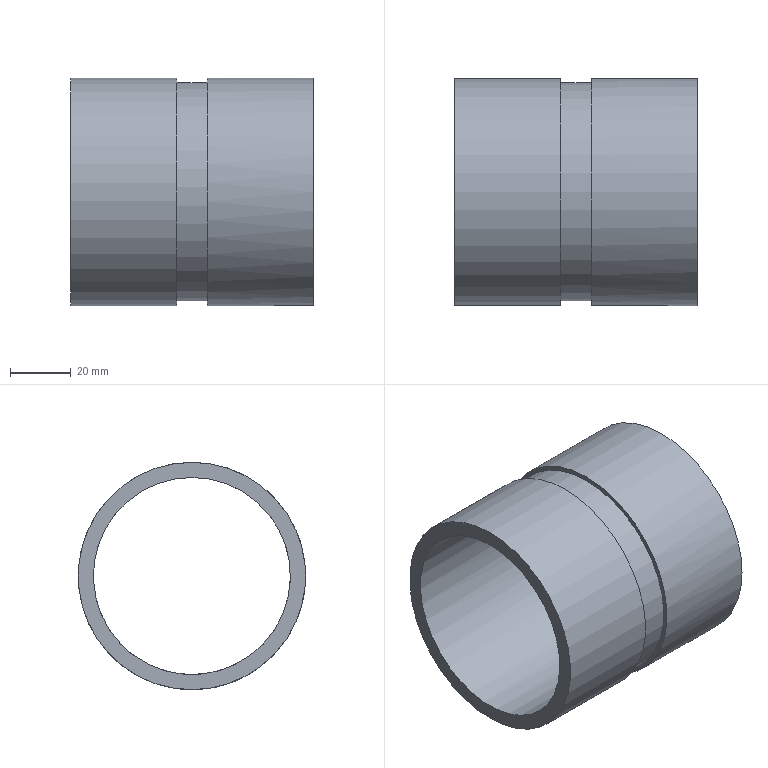Part | STEP file | gslz 2016.10.28-13_id442_x_t | 1 solid | 8 faces | box 80 x 75 x 75 mm | volume 84501 mm3 | cylinder 4 | plane 4 | commonest cylinder face diameters 75 x2 65 x1 72 x1
STEP:
#1=CARTESIAN_POINT('',(0.,0.,0.));
#2=DIRECTION('',(0.,0.,1.));
#3=DIRECTION('',(1.,0.,0.));
#4=AXIS2_PLACEMENT_3D('',#1,#2,#3);
#5=CARTESIAN_POINT('',(-1095.,-690.,260.5));
#6=VERTEX_POINT('',#5);
#7=CARTESIAN_POINT('',(-1095.,-690.,223.));
#8=DIRECTION('',(-1.,0.,0.));
#9=DIRECTION('',(0.,0.,1.));
#10=AXIS2_PLACEMENT_3D('',#7,#8,#9);
#11=CIRCLE('',#10,37.5);
#12=CARTESIAN_POINT('',(-1140.,-690.,223.));
#13=DIRECTION('',(1.,0.,0.));
#14=DIRECTION('',(0.,0.,1.));
#15=AXIS2_PLACEMENT_3D('',#12,#13,#14);
#16=CYLINDRICAL_SURFACE('',#15,37.5);
#17=CARTESIAN_POINT('',(6.283,45.));
#18=DIRECTION('',(-1.,0.));
#19=VECTOR('',#18,1.);
#20=LINE('',#17,#19);
#21=(GEOMETRIC_REPRESENTATION_CONTEXT(2)PARAMETRIC_REPRESENTATION_CONTEXT()REPRESENTATION_CONTEXT('',''));
#22=DEFINITIONAL_REPRESENTATION('',(#20),#21);
#23=PCURVE('',#16,#22);
#24=CARTESIAN_POINT('',(-1095.,-690.,223.));
#25=DIRECTION('',(1.,0.,0.));
#26=DIRECTION('',(0.,0.,1.));
#27=AXIS2_PLACEMENT_3D('',#24,#25,#26);
#28=PLANE('',#27);
#29=CARTESIAN_POINT('',(37.5,0.));
#30=CARTESIAN_POINT('',(37.5,-64.952));
#31=CARTESIAN_POINT('',(-18.75,-32.476));
#32=CARTESIAN_POINT('',(-75.,0.));
#33=CARTESIAN_POINT('',(-18.75,32.476));
#34=CARTESIAN_POINT('',(37.5,64.952));
#35=CARTESIAN_POINT('',(37.5,0.));
#36=(BOUNDED_CURVE()B_SPLINE_CURVE(2,(#29,#30,#31,#32,#33,#34,#35),.UNSPECIFIED.,.T.,.F.)B_SPLINE_CURVE_WITH_KNOTS((1,2,2,2,2,1),(-2.094,0.,2.094,4.189,6.283,8.378),.UNSPECIFIED.)CURVE()GEOMETRIC_REPRESENTATION_ITEM()RATIONAL_B_SPLINE_CURVE((1.,0.5,1.,0.5,1.,0.5,1.))REPRESENTATION_ITEM(''));
#37=(GEOMETRIC_REPRESENTATION_CONTEXT(2)PARAMETRIC_REPRESENTATION_CONTEXT()REPRESENTATION_CONTEXT('',''));
#38=DEFINITIONAL_REPRESENTATION('',(#36),#37);
#39=PCURVE('',#28,#38);
#40=SURFACE_CURVE('',#11,(#23,#39),.PCURVE_S1.);
#41=EDGE_CURVE('',#6,#6,#40,.T.);
#42=ORIENTED_EDGE('',*,*,#41,.F.);
#43=CARTESIAN_POINT('',(-1060.,-690.,260.5));
#44=VERTEX_POINT('',#43);
#45=CARTESIAN_POINT('',(-1095.,-690.,260.5));
#46=CARTESIAN_POINT('',(-1060.,-690.,260.5));
#47=B_SPLINE_CURVE_WITH_KNOTS('',1,(#45,#46),.UNSPECIFIED.,.F.,.F.,(2,2),(45.,80.),.PIECEWISE_BEZIER_KNOTS.);
#48=CARTESIAN_POINT('',(6.283,0.));
#49=DIRECTION('',(0.,1.));
#50=VECTOR('',#49,1.);
#51=LINE('',#48,#50);
#52=(GEOMETRIC_REPRESENTATION_CONTEXT(2)PARAMETRIC_REPRESENTATION_CONTEXT()REPRESENTATION_CONTEXT('',''));
#53=DEFINITIONAL_REPRESENTATION('',(#51),#52);
#54=PCURVE('',#16,#53);
#55=CARTESIAN_POINT('',(0.,0.));
#56=DIRECTION('',(0.,1.));
#57=VECTOR('',#56,1.);
#58=LINE('',#55,#57);
#59=(GEOMETRIC_REPRESENTATION_CONTEXT(2)PARAMETRIC_REPRESENTATION_CONTEXT()REPRESENTATION_CONTEXT('',''));
#60=DEFINITIONAL_REPRESENTATION('',(#58),#59);
#61=PCURVE('',#16,#60);
#62=SEAM_CURVE('',#47,(#54,#61),.PCURVE_S1.);
#63=EDGE_CURVE('',#6,#44,#62,.T.);
#64=ORIENTED_EDGE('',*,*,#63,.T.);
#65=CARTESIAN_POINT('',(-1060.,-727.5,223.));
#66=VERTEX_POINT('',#65);
#67=CARTESIAN_POINT('',(-1060.,-690.,223.));
#68=DIRECTION('',(-1.,0.,0.));
#69=DIRECTION('',(0.,-1.,0.));
#70=AXIS2_PLACEMENT_3D('',#67,#68,#69);
#71=CIRCLE('',#70,37.5);
#72=CARTESIAN_POINT('',(7.854,80.));
#73=DIRECTION('',(-1.,0.));
#74=VECTOR('',#73,1.);
#75=LINE('',#72,#74);
#76=(GEOMETRIC_REPRESENTATION_CONTEXT(2)PARAMETRIC_REPRESENTATION_CONTEXT()REPRESENTATION_CONTEXT('',''));
#77=DEFINITIONAL_REPRESENTATION('',(#75),#76);
#78=PCURVE('',#16,#77);
#79=CARTESIAN_POINT('',(-1060.,-585.,179.));
#80=DIRECTION('',(-1.,0.,0.));
#81=DIRECTION('',(0.,1.,0.));
#82=AXIS2_PLACEMENT_3D('',#79,#80,#81);
#83=PLANE('',#82);
#84=CARTESIAN_POINT('',(-105.,-44.));
#85=DIRECTION('',(-1.,0.));
#86=AXIS2_PLACEMENT_2D('',#84,#85);
#87=CIRCLE('',#86,37.5);
#88=(GEOMETRIC_REPRESENTATION_CONTEXT(2)PARAMETRIC_REPRESENTATION_CONTEXT()REPRESENTATION_CONTEXT('',''));
#89=DEFINITIONAL_REPRESENTATION('',(#87),#88);
#90=PCURVE('',#83,#89);
#91=SURFACE_CURVE('',#71,(#78,#90),.PCURVE_S1.);
#92=EDGE_CURVE('',#44,#66,#91,.T.);
#93=ORIENTED_EDGE('',*,*,#92,.T.);
#94=CARTESIAN_POINT('',(-1060.,-690.,223.));
#95=DIRECTION('',(-1.,0.,0.));
#96=DIRECTION('',(0.,-1.,0.));
#97=AXIS2_PLACEMENT_3D('',#94,#95,#96);
#98=CIRCLE('',#97,37.5);
#99=CARTESIAN_POINT('',(1.571,80.));
#100=DIRECTION('',(-1.,0.));
#101=VECTOR('',#100,1.);
#102=LINE('',#99,#101);
#103=(GEOMETRIC_REPRESENTATION_CONTEXT(2)PARAMETRIC_REPRESENTATION_CONTEXT()REPRESENTATION_CONTEXT('',''));
#104=DEFINITIONAL_REPRESENTATION('',(#102),#103);
#105=PCURVE('',#16,#104);
#106=CARTESIAN_POINT('',(-105.,-44.));
#107=DIRECTION('',(-1.,0.));
#108=AXIS2_PLACEMENT_2D('',#106,#107);
#109=CIRCLE('',#108,37.5);
#110=(GEOMETRIC_REPRESENTATION_CONTEXT(2)PARAMETRIC_REPRESENTATION_CONTEXT()REPRESENTATION_CONTEXT('',''));
#111=DEFINITIONAL_REPRESENTATION('',(#109),#110);
#112=PCURVE('',#83,#111);
#113=SURFACE_CURVE('',#98,(#105,#112),.PCURVE_S1.);
#114=EDGE_CURVE('',#66,#44,#113,.T.);
#115=ORIENTED_EDGE('',*,*,#114,.T.);
#116=ORIENTED_EDGE('',*,*,#63,.F.);
#117=EDGE_LOOP('',(#42,#64,#93,#115,#116));
#118=FACE_BOUND('',#117,.T.);
#119=ADVANCED_FACE('',(#118),#16,.T.);
#120=CARTESIAN_POINT('',(-1060.,-722.5,223.));
#121=VERTEX_POINT('',#120);
#122=CARTESIAN_POINT('',(-1060.,-690.,255.5));
#123=VERTEX_POINT('',#122);
#124=CARTESIAN_POINT('',(-1060.,-690.,223.));
#125=DIRECTION('',(-1.,0.,0.));
#126=DIRECTION('',(0.,-1.,0.));
#127=AXIS2_PLACEMENT_3D('',#124,#125,#126);
#128=CIRCLE('',#127,32.5);
#129=CARTESIAN_POINT('',(-105.,-44.));
#130=DIRECTION('',(-1.,0.));
#131=AXIS2_PLACEMENT_2D('',#129,#130);
#132=CIRCLE('',#131,32.5);
#133=(GEOMETRIC_REPRESENTATION_CONTEXT(2)PARAMETRIC_REPRESENTATION_CONTEXT()REPRESENTATION_CONTEXT('',''));
#134=DEFINITIONAL_REPRESENTATION('',(#132),#133);
#135=PCURVE('',#83,#134);
#136=CARTESIAN_POINT('',(-1140.,-690.,223.));
#137=DIRECTION('',(1.,0.,0.));
#138=DIRECTION('',(0.,0.,1.));
#139=AXIS2_PLACEMENT_3D('',#136,#137,#138);
#140=CYLINDRICAL_SURFACE('',#139,32.5);
#141=CARTESIAN_POINT('',(1.571,80.));
#142=DIRECTION('',(-1.,0.));
#143=VECTOR('',#142,1.);
#144=LINE('',#141,#143);
#145=(GEOMETRIC_REPRESENTATION_CONTEXT(2)PARAMETRIC_REPRESENTATION_CONTEXT()REPRESENTATION_CONTEXT('',''));
#146=DEFINITIONAL_REPRESENTATION('',(#144),#145);
#147=PCURVE('',#140,#146);
#148=SURFACE_CURVE('',#128,(#135,#147),.PCURVE_S1.);
#149=EDGE_CURVE('',#121,#123,#148,.T.);
#150=ORIENTED_EDGE('',*,*,#149,.T.);
#151=CARTESIAN_POINT('',(-1060.,-690.,223.));
#152=DIRECTION('',(-1.,0.,0.));
#153=DIRECTION('',(0.,-1.,0.));
#154=AXIS2_PLACEMENT_3D('',#151,#152,#153);
#155=CIRCLE('',#154,32.5);
#156=CARTESIAN_POINT('',(-105.,-44.));
#157=DIRECTION('',(-1.,0.));
#158=AXIS2_PLACEMENT_2D('',#156,#157);
#159=CIRCLE('',#158,32.5);
#160=(GEOMETRIC_REPRESENTATION_CONTEXT(2)PARAMETRIC_REPRESENTATION_CONTEXT()REPRESENTATION_CONTEXT('',''));
#161=DEFINITIONAL_REPRESENTATION('',(#159),#160);
#162=PCURVE('',#83,#161);
#163=CARTESIAN_POINT('',(7.854,80.));
#164=DIRECTION('',(-1.,0.));
#165=VECTOR('',#164,1.);
#166=LINE('',#163,#165);
#167=(GEOMETRIC_REPRESENTATION_CONTEXT(2)PARAMETRIC_REPRESENTATION_CONTEXT()REPRESENTATION_CONTEXT('',''));
#168=DEFINITIONAL_REPRESENTATION('',(#166),#167);
#169=PCURVE('',#140,#168);
#170=SURFACE_CURVE('',#155,(#162,#169),.PCURVE_S1.);
#171=EDGE_CURVE('',#123,#121,#170,.T.);
#172=ORIENTED_EDGE('',*,*,#171,.T.);
#173=EDGE_LOOP('',(#150,#172));
#174=FACE_BOUND('',#173,.T.);
#175=ORIENTED_EDGE('',*,*,#114,.F.);
#176=ORIENTED_EDGE('',*,*,#92,.F.);
#177=EDGE_LOOP('',(#175,#176));
#178=FACE_BOUND('',#177,.T.);
#179=ADVANCED_FACE('',(#174,#178),#83,.F.);
#180=CARTESIAN_POINT('',(-1140.,-690.,255.5));
#181=VERTEX_POINT('',#180);
#182=CARTESIAN_POINT('',(-1140.,-690.,223.));
#183=DIRECTION('',(1.,0.,0.));
#184=DIRECTION('',(0.,0.,1.));
#185=AXIS2_PLACEMENT_3D('',#182,#183,#184);
#186=CIRCLE('',#185,32.5);
#187=CARTESIAN_POINT('',(-1140.,-690.,223.));
#188=DIRECTION('',(-1.,0.,0.));
#189=DIRECTION('',(0.,0.,-1.));
#190=AXIS2_PLACEMENT_3D('',#187,#188,#189);
#191=PLANE('',#190);
#192=CARTESIAN_POINT('',(-32.5,0.));
#193=CARTESIAN_POINT('',(-32.5,56.292));
#194=CARTESIAN_POINT('',(16.25,28.146));
#195=CARTESIAN_POINT('',(65.,0.));
#196=CARTESIAN_POINT('',(16.25,-28.146));
#197=CARTESIAN_POINT('',(-32.5,-56.292));
#198=CARTESIAN_POINT('',(-32.5,0.));
#199=(BOUNDED_CURVE()B_SPLINE_CURVE(2,(#192,#193,#194,#195,#196,#197,#198),.UNSPECIFIED.,.T.,.F.)B_SPLINE_CURVE_WITH_KNOTS((1,2,2,2,2,1),(-2.094,0.,2.094,4.189,6.283,8.378),.UNSPECIFIED.)CURVE()GEOMETRIC_REPRESENTATION_ITEM()RATIONAL_B_SPLINE_CURVE((1.,0.5,1.,0.5,1.,0.5,1.))REPRESENTATION_ITEM(''));
#200=(GEOMETRIC_REPRESENTATION_CONTEXT(2)PARAMETRIC_REPRESENTATION_CONTEXT()REPRESENTATION_CONTEXT('',''));
#201=DEFINITIONAL_REPRESENTATION('',(#199),#200);
#202=PCURVE('',#191,#201);
#203=CARTESIAN_POINT('',(0.,0.));
#204=DIRECTION('',(1.,0.));
#205=VECTOR('',#204,1.);
#206=LINE('',#203,#205);
#207=(GEOMETRIC_REPRESENTATION_CONTEXT(2)PARAMETRIC_REPRESENTATION_CONTEXT()REPRESENTATION_CONTEXT('',''));
#208=DEFINITIONAL_REPRESENTATION('',(#206),#207);
#209=PCURVE('',#140,#208);
#210=SURFACE_CURVE('',#186,(#202,#209),.PCURVE_S1.);
#211=EDGE_CURVE('',#181,#181,#210,.T.);
#212=ORIENTED_EDGE('',*,*,#211,.T.);
#213=EDGE_LOOP('',(#212));
#214=FACE_BOUND('',#213,.T.);
#215=CARTESIAN_POINT('',(-1140.,-690.,260.5));
#216=VERTEX_POINT('',#215);
#217=CARTESIAN_POINT('',(-1140.,-690.,223.));
#218=DIRECTION('',(1.,0.,0.));
#219=DIRECTION('',(0.,0.,1.));
#220=AXIS2_PLACEMENT_3D('',#217,#218,#219);
#221=CIRCLE('',#220,37.5);
#222=CARTESIAN_POINT('',(-37.5,0.));
#223=CARTESIAN_POINT('',(-37.5,64.952));
#224=CARTESIAN_POINT('',(18.75,32.476));
#225=CARTESIAN_POINT('',(75.,0.));
#226=CARTESIAN_POINT('',(18.75,-32.476));
#227=CARTESIAN_POINT('',(-37.5,-64.952));
#228=CARTESIAN_POINT('',(-37.5,0.));
#229=(BOUNDED_CURVE()B_SPLINE_CURVE(2,(#222,#223,#224,#225,#226,#227,#228),.UNSPECIFIED.,.T.,.F.)B_SPLINE_CURVE_WITH_KNOTS((1,2,2,2,2,1),(-2.094,0.,2.094,4.189,6.283,8.378),.UNSPECIFIED.)CURVE()GEOMETRIC_REPRESENTATION_ITEM()RATIONAL_B_SPLINE_CURVE((1.,0.5,1.,0.5,1.,0.5,1.))REPRESENTATION_ITEM(''));
#230=(GEOMETRIC_REPRESENTATION_CONTEXT(2)PARAMETRIC_REPRESENTATION_CONTEXT()REPRESENTATION_CONTEXT('',''));
#231=DEFINITIONAL_REPRESENTATION('',(#229),#230);
#232=PCURVE('',#191,#231);
#233=CARTESIAN_POINT('',(-1140.,-690.,223.));
#234=DIRECTION('',(1.,0.,0.));
#235=DIRECTION('',(0.,0.,1.));
#236=AXIS2_PLACEMENT_3D('',#233,#234,#235);
#237=CYLINDRICAL_SURFACE('',#236,37.5);
#238=CARTESIAN_POINT('',(0.,0.));
#239=DIRECTION('',(1.,0.));
#240=VECTOR('',#239,1.);
#241=LINE('',#238,#240);
#242=(GEOMETRIC_REPRESENTATION_CONTEXT(2)PARAMETRIC_REPRESENTATION_CONTEXT()REPRESENTATION_CONTEXT('',''));
#243=DEFINITIONAL_REPRESENTATION('',(#241),#242);
#244=PCURVE('',#237,#243);
#245=SURFACE_CURVE('',#221,(#232,#244),.PCURVE_S1.);
#246=EDGE_CURVE('',#216,#216,#245,.T.);
#247=ORIENTED_EDGE('',*,*,#246,.F.);
#248=EDGE_LOOP('',(#247));
#249=FACE_BOUND('',#248,.T.);
#250=ADVANCED_FACE('',(#214,#249),#191,.T.);
#251=CARTESIAN_POINT('',(-1105.,-690.,260.5));
#252=VERTEX_POINT('',#251);
#253=CARTESIAN_POINT('',(-1105.,-690.,223.));
#254=DIRECTION('',(1.,0.,0.));
#255=DIRECTION('',(0.,0.,1.));
#256=AXIS2_PLACEMENT_3D('',#253,#254,#255);
#257=CIRCLE('',#256,37.5);
#258=CARTESIAN_POINT('',(0.,35.));
#259=DIRECTION('',(1.,0.));
#260=VECTOR('',#259,1.);
#261=LINE('',#258,#260);
#262=(GEOMETRIC_REPRESENTATION_CONTEXT(2)PARAMETRIC_REPRESENTATION_CONTEXT()REPRESENTATION_CONTEXT('',''));
#263=DEFINITIONAL_REPRESENTATION('',(#261),#262);
#264=PCURVE('',#237,#263);
#265=CARTESIAN_POINT('',(-1105.,-690.,223.));
#266=DIRECTION('',(-1.,0.,0.));
#267=DIRECTION('',(0.,0.,-1.));
#268=AXIS2_PLACEMENT_3D('',#265,#266,#267);
#269=PLANE('',#268);
#270=CARTESIAN_POINT('',(-37.5,0.));
#271=CARTESIAN_POINT('',(-37.5,64.952));
#272=CARTESIAN_POINT('',(18.75,32.476));
#273=CARTESIAN_POINT('',(75.,0.));
#274=CARTESIAN_POINT('',(18.75,-32.476));
#275=CARTESIAN_POINT('',(-37.5,-64.952));
#276=CARTESIAN_POINT('',(-37.5,0.));
#277=(BOUNDED_CURVE()B_SPLINE_CURVE(2,(#270,#271,#272,#273,#274,#275,#276),.UNSPECIFIED.,.T.,.F.)B_SPLINE_CURVE_WITH_KNOTS((1,2,2,2,2,1),(-2.094,0.,2.094,4.189,6.283,8.378),.UNSPECIFIED.)CURVE()GEOMETRIC_REPRESENTATION_ITEM()RATIONAL_B_SPLINE_CURVE((1.,0.5,1.,0.5,1.,0.5,1.))REPRESENTATION_ITEM(''));
#278=(GEOMETRIC_REPRESENTATION_CONTEXT(2)PARAMETRIC_REPRESENTATION_CONTEXT()REPRESENTATION_CONTEXT('',''));
#279=DEFINITIONAL_REPRESENTATION('',(#277),#278);
#280=PCURVE('',#269,#279);
#281=SURFACE_CURVE('',#257,(#264,#280),.PCURVE_S1.);
#282=EDGE_CURVE('',#252,#252,#281,.T.);
#283=ORIENTED_EDGE('',*,*,#282,.F.);
#284=CARTESIAN_POINT('',(-1140.,-690.,260.5));
#285=CARTESIAN_POINT('',(-1105.,-690.,260.5));
#286=B_SPLINE_CURVE_WITH_KNOTS('',1,(#284,#285),.UNSPECIFIED.,.F.,.F.,(2,2),(0.,35.),.PIECEWISE_BEZIER_KNOTS.);
#287=CARTESIAN_POINT('',(0.,0.));
#288=DIRECTION('',(0.,1.));
#289=VECTOR('',#288,1.);
#290=LINE('',#287,#289);
#291=(GEOMETRIC_REPRESENTATION_CONTEXT(2)PARAMETRIC_REPRESENTATION_CONTEXT()REPRESENTATION_CONTEXT('',''));
#292=DEFINITIONAL_REPRESENTATION('',(#290),#291);
#293=PCURVE('',#237,#292);
#294=CARTESIAN_POINT('',(6.283,0.));
#295=DIRECTION('',(0.,1.));
#296=VECTOR('',#295,1.);
#297=LINE('',#294,#296);
#298=(GEOMETRIC_REPRESENTATION_CONTEXT(2)PARAMETRIC_REPRESENTATION_CONTEXT()REPRESENTATION_CONTEXT('',''));
#299=DEFINITIONAL_REPRESENTATION('',(#297),#298);
#300=PCURVE('',#237,#299);
#301=SEAM_CURVE('',#286,(#293,#300),.PCURVE_S1.);
#302=EDGE_CURVE('',#216,#252,#301,.T.);
#303=ORIENTED_EDGE('',*,*,#302,.F.);
#304=ORIENTED_EDGE('',*,*,#246,.T.);
#305=ORIENTED_EDGE('',*,*,#302,.T.);
#306=EDGE_LOOP('',(#283,#303,#304,#305));
#307=FACE_BOUND('',#306,.T.);
#308=ADVANCED_FACE('',(#307),#237,.T.);
#309=ORIENTED_EDGE('',*,*,#149,.T.);
#310=CARTESIAN_POINT('',(-1140.,-690.,255.5));
#311=CARTESIAN_POINT('',(-1060.,-690.,255.5));
#312=B_SPLINE_CURVE_WITH_KNOTS('',1,(#310,#311),.UNSPECIFIED.,.F.,.F.,(2,2),(0.,80.),.PIECEWISE_BEZIER_KNOTS.);
#313=CARTESIAN_POINT('',(0.,0.));
#314=DIRECTION('',(0.,1.));
#315=VECTOR('',#314,1.);
#316=LINE('',#313,#315);
#317=(GEOMETRIC_REPRESENTATION_CONTEXT(2)PARAMETRIC_REPRESENTATION_CONTEXT()REPRESENTATION_CONTEXT('',''));
#318=DEFINITIONAL_REPRESENTATION('',(#316),#317);
#319=PCURVE('',#140,#318);
#320=CARTESIAN_POINT('',(6.283,0.));
#321=DIRECTION('',(0.,1.));
#322=VECTOR('',#321,1.);
#323=LINE('',#320,#322);
#324=(GEOMETRIC_REPRESENTATION_CONTEXT(2)PARAMETRIC_REPRESENTATION_CONTEXT()REPRESENTATION_CONTEXT('',''));
#325=DEFINITIONAL_REPRESENTATION('',(#323),#324);
#326=PCURVE('',#140,#325);
#327=SEAM_CURVE('',#312,(#319,#326),.PCURVE_S1.);
#328=EDGE_CURVE('',#181,#123,#327,.T.);
#329=ORIENTED_EDGE('',*,*,#328,.F.);
#330=ORIENTED_EDGE('',*,*,#211,.T.);
#331=ORIENTED_EDGE('',*,*,#328,.T.);
#332=ORIENTED_EDGE('',*,*,#171,.T.);
#333=EDGE_LOOP('',(#309,#329,#330,#331,#332));
#334=FACE_BOUND('',#333,.F.);
#335=ADVANCED_FACE('',(#334),#140,.F.);
#336=CARTESIAN_POINT('',(-1095.,-690.,259.));
#337=VERTEX_POINT('',#336);
#338=CARTESIAN_POINT('',(-1095.,-690.,223.));
#339=DIRECTION('',(1.,0.,0.));
#340=DIRECTION('',(0.,0.,1.));
#341=AXIS2_PLACEMENT_3D('',#338,#339,#340);
#342=CIRCLE('',#341,36.);
#343=CARTESIAN_POINT('',(0.,0.));
#344=DIRECTION('',(1.,0.));
#345=AXIS2_PLACEMENT_2D('',#343,#344);
#346=CIRCLE('',#345,36.);
#347=(GEOMETRIC_REPRESENTATION_CONTEXT(2)PARAMETRIC_REPRESENTATION_CONTEXT()REPRESENTATION_CONTEXT('',''));
#348=DEFINITIONAL_REPRESENTATION('',(#346),#347);
#349=PCURVE('',#28,#348);
#350=CARTESIAN_POINT('',(-1105.,-690.,223.));
#351=DIRECTION('',(1.,0.,0.));
#352=DIRECTION('',(0.,0.,1.));
#353=AXIS2_PLACEMENT_3D('',#350,#351,#352);
#354=CYLINDRICAL_SURFACE('',#353,36.);
#355=CARTESIAN_POINT('',(0.,10.));
#356=DIRECTION('',(1.,0.));
#357=VECTOR('',#356,1.);
#358=LINE('',#355,#357);
#359=(GEOMETRIC_REPRESENTATION_CONTEXT(2)PARAMETRIC_REPRESENTATION_CONTEXT()REPRESENTATION_CONTEXT('',''));
#360=DEFINITIONAL_REPRESENTATION('',(#358),#359);
#361=PCURVE('',#354,#360);
#362=SURFACE_CURVE('',#342,(#349,#361),.PCURVE_S1.);
#363=EDGE_CURVE('',#337,#337,#362,.T.);
#364=ORIENTED_EDGE('',*,*,#363,.T.);
#365=EDGE_LOOP('',(#364));
#366=FACE_BOUND('',#365,.T.);
#367=ORIENTED_EDGE('',*,*,#41,.T.);
#368=EDGE_LOOP('',(#367));
#369=FACE_BOUND('',#368,.T.);
#370=ADVANCED_FACE('',(#366,#369),#28,.F.);
#371=CARTESIAN_POINT('',(-1105.,-690.,259.));
#372=VERTEX_POINT('',#371);
#373=CARTESIAN_POINT('',(-1105.,-690.,223.));
#374=DIRECTION('',(-1.,0.,0.));
#375=DIRECTION('',(0.,0.,1.));
#376=AXIS2_PLACEMENT_3D('',#373,#374,#375);
#377=CIRCLE('',#376,36.);
#378=CARTESIAN_POINT('',(0.,0.));
#379=DIRECTION('',(-1.,0.));
#380=AXIS2_PLACEMENT_2D('',#378,#379);
#381=CIRCLE('',#380,36.);
#382=(GEOMETRIC_REPRESENTATION_CONTEXT(2)PARAMETRIC_REPRESENTATION_CONTEXT()REPRESENTATION_CONTEXT('',''));
#383=DEFINITIONAL_REPRESENTATION('',(#381),#382);
#384=PCURVE('',#269,#383);
#385=CARTESIAN_POINT('',(6.283,0.));
#386=DIRECTION('',(-1.,0.));
#387=VECTOR('',#386,1.);
#388=LINE('',#385,#387);
#389=(GEOMETRIC_REPRESENTATION_CONTEXT(2)PARAMETRIC_REPRESENTATION_CONTEXT()REPRESENTATION_CONTEXT('',''));
#390=DEFINITIONAL_REPRESENTATION('',(#388),#389);
#391=PCURVE('',#354,#390);
#392=SURFACE_CURVE('',#377,(#384,#391),.PCURVE_S1.);
#393=EDGE_CURVE('',#372,#372,#392,.T.);
#394=ORIENTED_EDGE('',*,*,#393,.T.);
#395=EDGE_LOOP('',(#394));
#396=FACE_BOUND('',#395,.T.);
#397=ORIENTED_EDGE('',*,*,#282,.T.);
#398=EDGE_LOOP('',(#397));
#399=FACE_BOUND('',#398,.T.);
#400=ADVANCED_FACE('',(#396,#399),#269,.F.);
#401=ORIENTED_EDGE('',*,*,#363,.F.);
#402=CARTESIAN_POINT('',(-1105.,-690.,259.));
#403=CARTESIAN_POINT('',(-1095.,-690.,259.));
#404=B_SPLINE_CURVE_WITH_KNOTS('',1,(#402,#403),.UNSPECIFIED.,.F.,.F.,(2,2),(0.,10.),.PIECEWISE_BEZIER_KNOTS.);
#405=CARTESIAN_POINT('',(0.,0.));
#406=DIRECTION('',(0.,1.));
#407=VECTOR('',#406,1.);
#408=LINE('',#405,#407);
#409=(GEOMETRIC_REPRESENTATION_CONTEXT(2)PARAMETRIC_REPRESENTATION_CONTEXT()REPRESENTATION_CONTEXT('',''));
#410=DEFINITIONAL_REPRESENTATION('',(#408),#409);
#411=PCURVE('',#354,#410);
#412=CARTESIAN_POINT('',(6.283,0.));
#413=DIRECTION('',(0.,1.));
#414=VECTOR('',#413,1.);
#415=LINE('',#412,#414);
#416=(GEOMETRIC_REPRESENTATION_CONTEXT(2)PARAMETRIC_REPRESENTATION_CONTEXT()REPRESENTATION_CONTEXT('',''));
#417=DEFINITIONAL_REPRESENTATION('',(#415),#416);
#418=PCURVE('',#354,#417);
#419=SEAM_CURVE('',#404,(#411,#418),.PCURVE_S1.);
#420=EDGE_CURVE('',#372,#337,#419,.T.);
#421=ORIENTED_EDGE('',*,*,#420,.F.);
#422=ORIENTED_EDGE('',*,*,#393,.F.);
#423=ORIENTED_EDGE('',*,*,#420,.T.);
#424=EDGE_LOOP('',(#401,#421,#422,#423));
#425=FACE_BOUND('',#424,.T.);
#426=ADVANCED_FACE('',(#425),#354,.T.);
#427=CLOSED_SHELL('',(#119,#179,#250,#308,#335,#370,#400,#426));
#428=MANIFOLD_SOLID_BREP('',#427);
#429=(LENGTH_UNIT()NAMED_UNIT(*)SI_UNIT(.MILLI.,.METRE.));
#430=UNCERTAINTY_MEASURE_WITH_UNIT(LENGTH_MEASURE(0.000005),#429,'','');
#431=(NAMED_UNIT(*)PLANE_ANGLE_UNIT()SI_UNIT($,.RADIAN.));
#432=(NAMED_UNIT(*)SI_UNIT($,.STERADIAN.)SOLID_ANGLE_UNIT());
#433=(GEOMETRIC_REPRESENTATION_CONTEXT(3)GLOBAL_UNCERTAINTY_ASSIGNED_CONTEXT((#430))GLOBAL_UNIT_ASSIGNED_CONTEXT((#429,#431,#432))REPRESENTATION_CONTEXT('',''));
#434=ADVANCED_BREP_SHAPE_REPRESENTATION('',(#4,#428),#433);